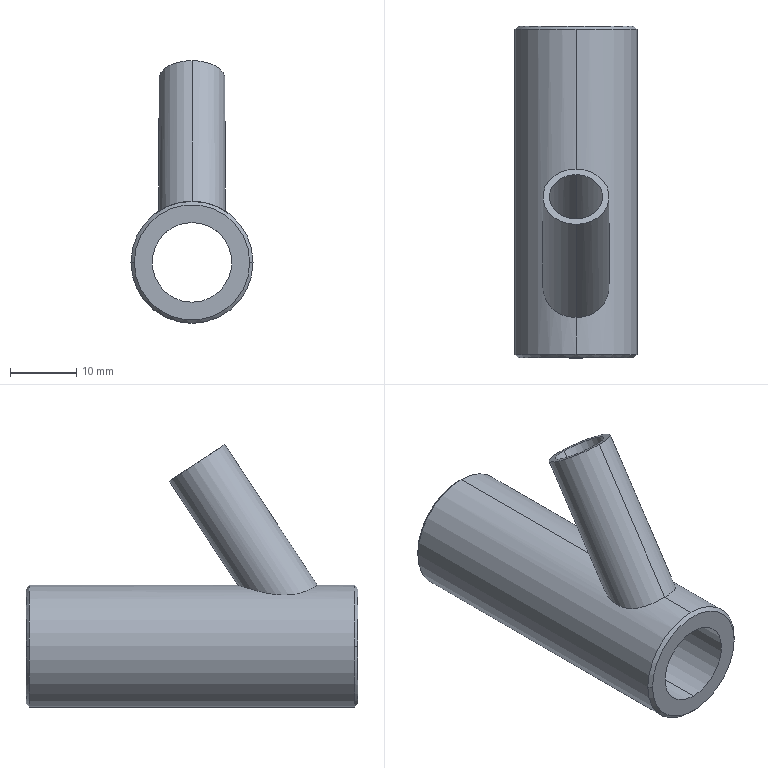Part | STEP file | fBY012F01M-03-02A | 1 solid | 18 faces | box 18.4 x 50 x 39.602 mm | volume 7485 mm3 | cylinder 10 | cone 4 | plane 4 | commonest cylinder face diameters 8 x2 10 x2 12 x2 15.4 x2 18.4 x2